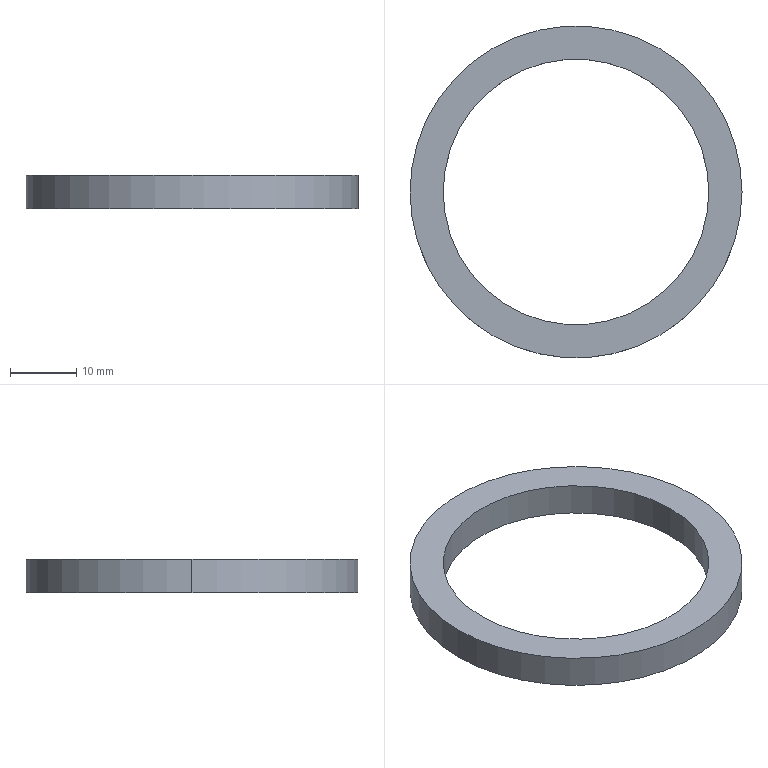Part | SolidWorks | features Extrusion 1 | 1 solid | 6 faces | box 50 x 50 x 5 mm | volume 3534 mm3 | cylinder 4 | plane 2 | commonest cylinder face diameters 40 x2 50 x2
STEP:
#1=CARTESIAN_POINT('',(-20.,0.,5.));
#2=VERTEX_POINT('',#1);
#3=CARTESIAN_POINT('',(20.,0.,5.));
#4=VERTEX_POINT('',#3);
#5=CARTESIAN_POINT('',(0.,0.,5.));
#6=DIRECTION('',(0.,0.,1.));
#7=DIRECTION('',(1.,0.,0.));
#8=AXIS2_PLACEMENT_3D('',#5,#6,#7);
#9=CIRCLE('',#8,20.);
#10=EDGE_CURVE('',#2,#4,#9,.T.);
#11=ORIENTED_EDGE('',*,*,#10,.T.);
#12=CARTESIAN_POINT('',(20.,0.,0.));
#13=VERTEX_POINT('',#12);
#14=CARTESIAN_POINT('',(20.,0.,5.));
#15=DIRECTION('',(0.,0.,-1.));
#16=VECTOR('',#15,1000.);
#17=LINE('',#14,#16);
#18=EDGE_CURVE('',#4,#13,#17,.T.);
#19=ORIENTED_EDGE('',*,*,#18,.T.);
#20=CARTESIAN_POINT('',(-20.,0.,0.));
#21=VERTEX_POINT('',#20);
#22=CARTESIAN_POINT('',(0.,0.,0.));
#23=DIRECTION('',(0.,0.,1.));
#24=DIRECTION('',(1.,0.,0.));
#25=AXIS2_PLACEMENT_3D('',#22,#23,#24);
#26=CIRCLE('',#25,20.);
#27=EDGE_CURVE('',#21,#13,#26,.T.);
#28=ORIENTED_EDGE('',*,*,#27,.F.);
#29=CARTESIAN_POINT('',(-20.,0.,5.));
#30=DIRECTION('',(0.,0.,-1.));
#31=VECTOR('',#30,1000.);
#32=LINE('',#29,#31);
#33=EDGE_CURVE('',#2,#21,#32,.T.);
#34=ORIENTED_EDGE('',*,*,#33,.F.);
#35=EDGE_LOOP('',(#11,#19,#28,#34));
#36=FACE_OUTER_BOUND('',#35,.T.);
#37=CARTESIAN_POINT('',(0.,0.,5.));
#38=DIRECTION('',(0.,0.,-1.));
#39=DIRECTION('',(-1.,0.,0.));
#40=AXIS2_PLACEMENT_3D('',#37,#38,#39);
#41=CYLINDRICAL_SURFACE('',#40,20.);
#42=ADVANCED_FACE('',(#36),#41,.F.);
#43=CARTESIAN_POINT('',(25.,0.,5.));
#44=VERTEX_POINT('',#43);
#45=CARTESIAN_POINT('',(-25.,0.,5.));
#46=VERTEX_POINT('',#45);
#47=CARTESIAN_POINT('',(0.,0.,5.));
#48=DIRECTION('',(0.,0.,1.));
#49=DIRECTION('',(1.,0.,0.));
#50=AXIS2_PLACEMENT_3D('',#47,#48,#49);
#51=CIRCLE('',#50,25.);
#52=EDGE_CURVE('',#44,#46,#51,.T.);
#53=ORIENTED_EDGE('',*,*,#52,.F.);
#54=CARTESIAN_POINT('',(25.,0.,0.));
#55=VERTEX_POINT('',#54);
#56=CARTESIAN_POINT('',(25.,0.,5.));
#57=DIRECTION('',(0.,0.,-1.));
#58=VECTOR('',#57,1000.);
#59=LINE('',#56,#58);
#60=EDGE_CURVE('',#44,#55,#59,.T.);
#61=ORIENTED_EDGE('',*,*,#60,.T.);
#62=CARTESIAN_POINT('',(-25.,0.,0.));
#63=VERTEX_POINT('',#62);
#64=CARTESIAN_POINT('',(0.,0.,0.));
#65=DIRECTION('',(0.,0.,1.));
#66=DIRECTION('',(1.,0.,0.));
#67=AXIS2_PLACEMENT_3D('',#64,#65,#66);
#68=CIRCLE('',#67,25.);
#69=EDGE_CURVE('',#55,#63,#68,.T.);
#70=ORIENTED_EDGE('',*,*,#69,.T.);
#71=CARTESIAN_POINT('',(-25.,0.,5.));
#72=DIRECTION('',(0.,0.,-1.));
#73=VECTOR('',#72,1000.);
#74=LINE('',#71,#73);
#75=EDGE_CURVE('',#46,#63,#74,.T.);
#76=ORIENTED_EDGE('',*,*,#75,.F.);
#77=EDGE_LOOP('',(#53,#61,#70,#76));
#78=FACE_OUTER_BOUND('',#77,.T.);
#79=CARTESIAN_POINT('',(0.,0.,5.));
#80=DIRECTION('',(0.,0.,-1.));
#81=DIRECTION('',(-1.,0.,0.));
#82=AXIS2_PLACEMENT_3D('',#79,#80,#81);
#83=CYLINDRICAL_SURFACE('',#82,25.);
#84=ADVANCED_FACE('',(#78),#83,.T.);
#85=CARTESIAN_POINT('',(0.,0.,5.));
#86=DIRECTION('',(0.,0.,1.));
#87=DIRECTION('',(1.,0.,0.));
#88=AXIS2_PLACEMENT_3D('',#85,#86,#87);
#89=CIRCLE('',#88,25.);
#90=EDGE_CURVE('',#46,#44,#89,.T.);
#91=ORIENTED_EDGE('',*,*,#90,.T.);
#92=ORIENTED_EDGE('',*,*,#52,.T.);
#93=EDGE_LOOP('',(#91,#92));
#94=FACE_OUTER_BOUND('',#93,.T.);
#95=ORIENTED_EDGE('',*,*,#10,.F.);
#96=CARTESIAN_POINT('',(0.,0.,5.));
#97=DIRECTION('',(0.,0.,1.));
#98=DIRECTION('',(1.,0.,0.));
#99=AXIS2_PLACEMENT_3D('',#96,#97,#98);
#100=CIRCLE('',#99,20.);
#101=EDGE_CURVE('',#4,#2,#100,.T.);
#102=ORIENTED_EDGE('',*,*,#101,.F.);
#103=EDGE_LOOP('',(#95,#102));
#104=FACE_BOUND('',#103,.T.);
#105=CARTESIAN_POINT('',(0.,0.,5.));
#106=DIRECTION('',(0.,0.,1.));
#107=DIRECTION('',(1.,0.,0.));
#108=AXIS2_PLACEMENT_3D('',#105,#106,#107);
#109=PLANE('',#108);
#110=ADVANCED_FACE('',(#94,#104),#109,.T.);
#111=CARTESIAN_POINT('',(0.,0.,0.));
#112=DIRECTION('',(0.,0.,1.));
#113=DIRECTION('',(1.,0.,0.));
#114=AXIS2_PLACEMENT_3D('',#111,#112,#113);
#115=CIRCLE('',#114,25.);
#116=EDGE_CURVE('',#63,#55,#115,.T.);
#117=ORIENTED_EDGE('',*,*,#116,.F.);
#118=ORIENTED_EDGE('',*,*,#69,.F.);
#119=EDGE_LOOP('',(#117,#118));
#120=FACE_OUTER_BOUND('',#119,.T.);
#121=ORIENTED_EDGE('',*,*,#27,.T.);
#122=CARTESIAN_POINT('',(0.,0.,0.));
#123=DIRECTION('',(0.,0.,1.));
#124=DIRECTION('',(1.,0.,0.));
#125=AXIS2_PLACEMENT_3D('',#122,#123,#124);
#126=CIRCLE('',#125,20.);
#127=EDGE_CURVE('',#13,#21,#126,.T.);
#128=ORIENTED_EDGE('',*,*,#127,.T.);
#129=EDGE_LOOP('',(#121,#128));
#130=FACE_BOUND('',#129,.T.);
#131=CARTESIAN_POINT('',(0.,0.,0.));
#132=DIRECTION('',(0.,0.,1.));
#133=DIRECTION('',(1.,0.,0.));
#134=AXIS2_PLACEMENT_3D('',#131,#132,#133);
#135=PLANE('',#134);
#136=ADVANCED_FACE('',(#120,#130),#135,.F.);
#137=ORIENTED_EDGE('',*,*,#60,.F.);
#138=ORIENTED_EDGE('',*,*,#90,.F.);
#139=ORIENTED_EDGE('',*,*,#75,.T.);
#140=ORIENTED_EDGE('',*,*,#116,.T.);
#141=EDGE_LOOP('',(#137,#138,#139,#140));
#142=FACE_OUTER_BOUND('',#141,.T.);
#143=CARTESIAN_POINT('',(0.,0.,5.));
#144=DIRECTION('',(0.,0.,-1.));
#145=DIRECTION('',(-1.,0.,0.));
#146=AXIS2_PLACEMENT_3D('',#143,#144,#145);
#147=CYLINDRICAL_SURFACE('',#146,25.);
#148=ADVANCED_FACE('',(#142),#147,.T.);
#149=ORIENTED_EDGE('',*,*,#18,.F.);
#150=ORIENTED_EDGE('',*,*,#101,.T.);
#151=ORIENTED_EDGE('',*,*,#33,.T.);
#152=ORIENTED_EDGE('',*,*,#127,.F.);
#153=EDGE_LOOP('',(#149,#150,#151,#152));
#154=FACE_OUTER_BOUND('',#153,.T.);
#155=CARTESIAN_POINT('',(0.,0.,5.));
#156=DIRECTION('',(0.,0.,-1.));
#157=DIRECTION('',(-1.,0.,0.));
#158=AXIS2_PLACEMENT_3D('',#155,#156,#157);
#159=CYLINDRICAL_SURFACE('',#158,20.);
#160=ADVANCED_FACE('',(#154),#159,.F.);
#161=CLOSED_SHELL('',(#42,#84,#110,#136,#148,#160));
#162=MANIFOLD_SOLID_BREP('',#161);
#163=CARTESIAN_POINT('',(0.,0.,0.));
#164=DIRECTION('',(0.,0.,1.));
#165=DIRECTION('',(1.,0.,0.));
#166=AXIS2_PLACEMENT_3D('',#163,#164,#165);
#167=(LENGTH_UNIT()NAMED_UNIT(*)SI_UNIT(.MILLI.,.METRE.));
#168=UNCERTAINTY_MEASURE_WITH_UNIT(LENGTH_MEASURE(0.00001),#167,'','');
#169=(NAMED_UNIT(*)PLANE_ANGLE_UNIT()SI_UNIT($,.RADIAN.));
#170=(NAMED_UNIT(*)SI_UNIT($,.STERADIAN.)SOLID_ANGLE_UNIT());
#171=(GEOMETRIC_REPRESENTATION_CONTEXT(3)GLOBAL_UNCERTAINTY_ASSIGNED_CONTEXT((#168))GLOBAL_UNIT_ASSIGNED_CONTEXT((#167,#169,#170))REPRESENTATION_CONTEXT('',''));
#172=ADVANCED_BREP_SHAPE_REPRESENTATION('',(#162,#166),#171);